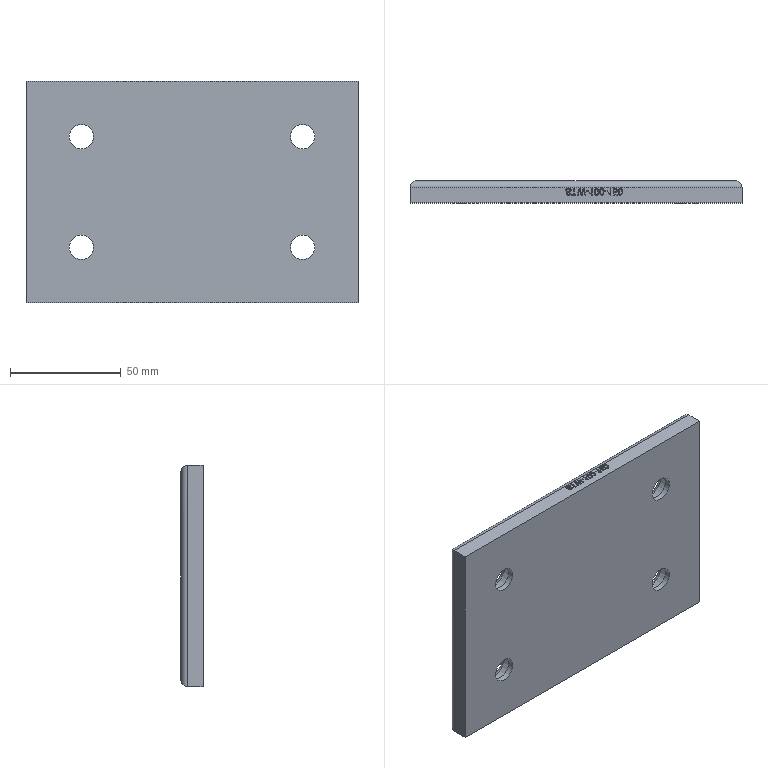Part | STEP file | lll_id5038_x_t | 1 solid | 111 faces | box 150 x 10 x 100 mm | volume 140671 mm3 | plane 66 | other 29 | cylinder 12 | torus 4 | commonest cylinder face diameters 6 x4 11 x4 17.5 x4